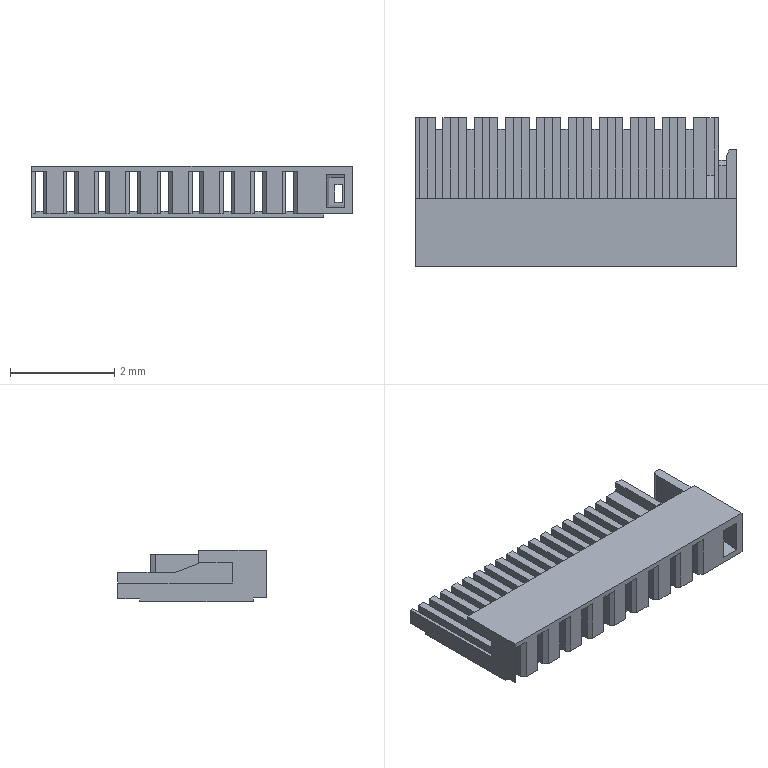Part | Creo | 1 solid | 270 faces | box 6.15 x 2.85 x 0.98 mm | volume 6.669 mm3 | plane 270